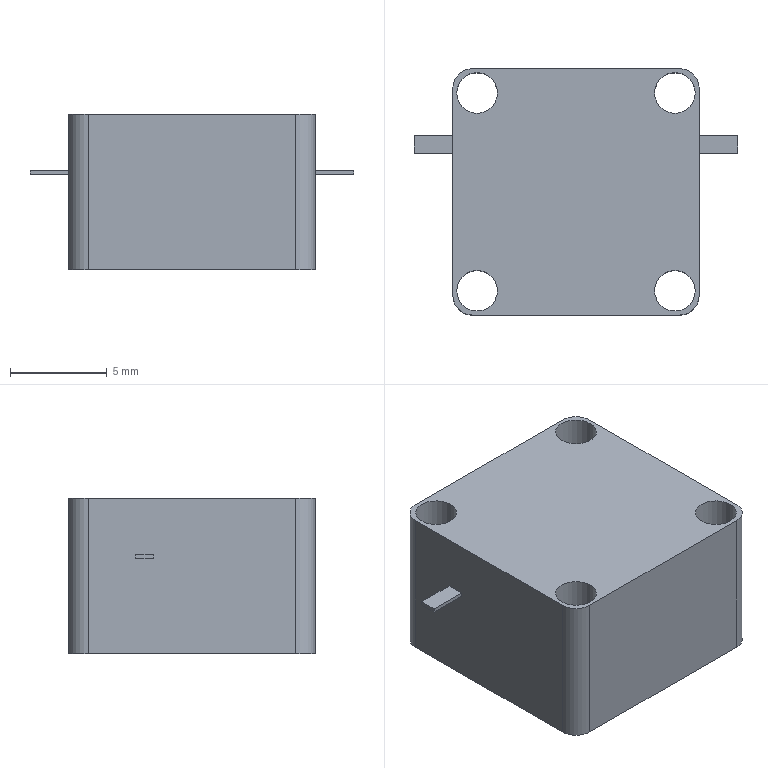Part | STEP file | UIYDI1212B5300T5900 | 2 solids | 107 faces | box 16.7 x 12.7 x 8 mm | volume 1173 mm3 | plane 54 | other 45 | cylinder 8 | commonest cylinder face diameters 2 x4 2.1 x4